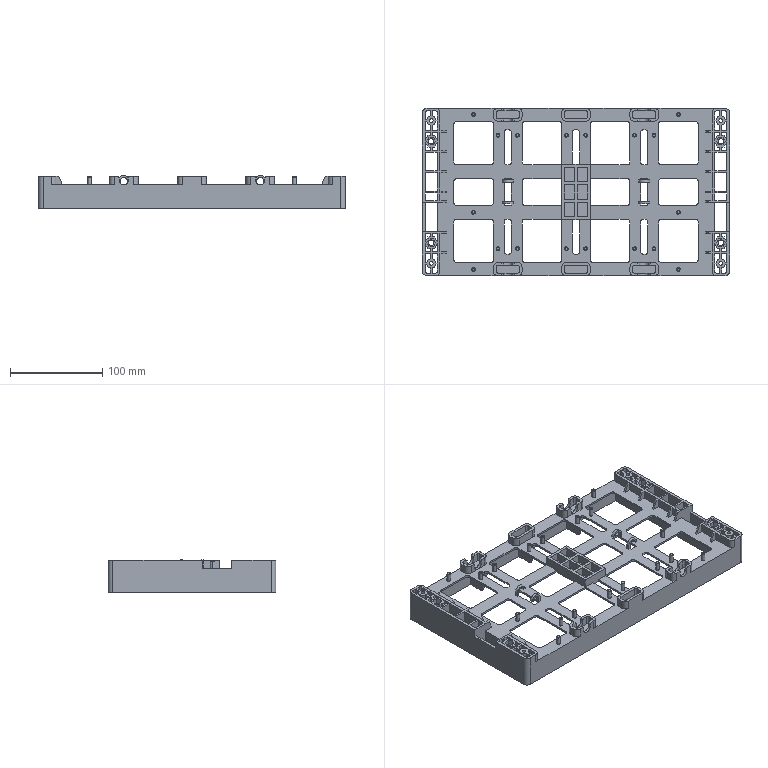Part | NX | features BREP 1 | 1 solid | 816 faces | box 333 x 182 x 35.5 mm | volume 244246 mm3 | plane 534 | cylinder 230 | cone 48 | torus 4 | commonest cylinder face diameters 4 x92 6 x68 10 x62 8 x4 12 x4